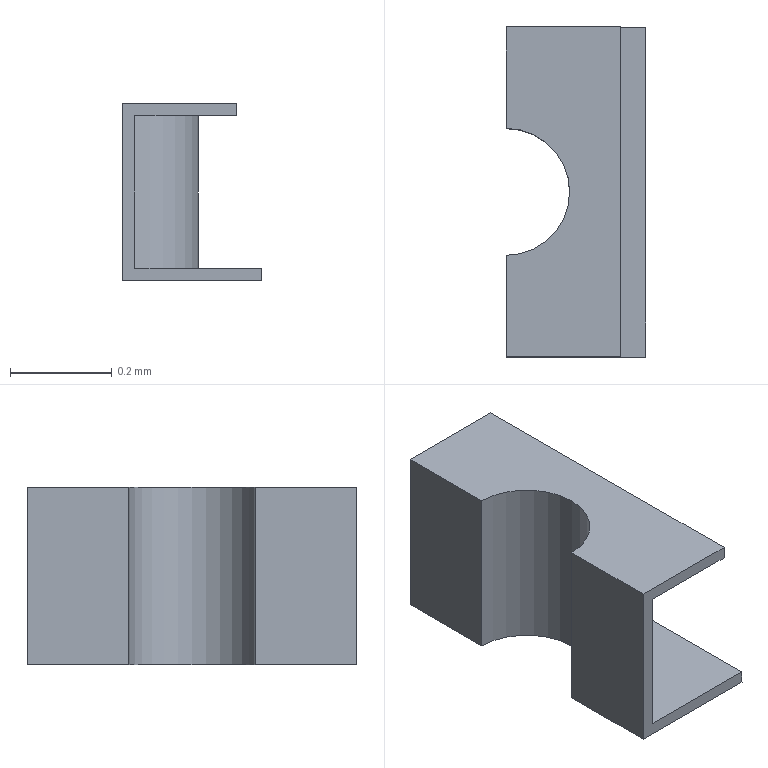Part | STEP file | RJ-USIO-V1_2-220411_91 | 1 solid | 14 faces | box 0.275 x 0.65 x 0.35 mm | volume 0.01277 mm3 | plane 12 | cylinder 2 | commonest cylinder face diameters 0.25 x1 0.3 x1
STEP:
#1=CARTESIAN_POINT('',(0.,0.,0.));
#2=DIRECTION('',(0.,0.,1.));
#3=DIRECTION('',(1.,0.,0.));
#4=AXIS2_PLACEMENT_3D('',#1,#2,#3);
#5=CARTESIAN_POINT('',(59.475,56.625,0.004766));
#6=VERTEX_POINT('',#5);
#7=CARTESIAN_POINT('',(59.475,56.825,0.004766));
#8=VERTEX_POINT('',#7);
#9=CARTESIAN_POINT('',(59.475,56.625,0.004766));
#10=DIRECTION('',(-0.000000044,1.,0.));
#11=VECTOR('',#10,1.);
#12=LINE('',#9,#11);
#13=CARTESIAN_POINT('',(59.55,56.5,0.004766));
#14=DIRECTION('',(0.,0.,1.));
#15=DIRECTION('',(0.000000044,-1.,0.));
#16=AXIS2_PLACEMENT_3D('',#13,#14,#15);
#17=PLANE('',#16);
#18=CARTESIAN_POINT('',(-0.125,-0.07522));
#19=DIRECTION('',(-1.,0.));
#20=VECTOR('',#19,1.);
#21=LINE('',#18,#20);
#22=(GEOMETRIC_REPRESENTATION_CONTEXT(2)PARAMETRIC_REPRESENTATION_CONTEXT()REPRESENTATION_CONTEXT('',''));
#23=DEFINITIONAL_REPRESENTATION('',(#21),#22);
#24=PCURVE('',#17,#23);
#25=CARTESIAN_POINT('',(59.475,56.65,0.004766));
#26=DIRECTION('',(-1.,-0.000000044,0.));
#27=DIRECTION('',(-0.000000044,1.,0.));
#28=AXIS2_PLACEMENT_3D('',#25,#26,#27);
#29=PLANE('',#28);
#30=CARTESIAN_POINT('',(-0.025,0.));
#31=DIRECTION('',(1.,0.));
#32=VECTOR('',#31,1.);
#33=LINE('',#30,#32);
#34=(GEOMETRIC_REPRESENTATION_CONTEXT(2)PARAMETRIC_REPRESENTATION_CONTEXT()REPRESENTATION_CONTEXT('',''));
#35=DEFINITIONAL_REPRESENTATION('',(#33),#34);
#36=PCURVE('',#29,#35);
#37=SURFACE_CURVE('',#12,(#24,#36),.PCURVE_S1.);
#38=EDGE_CURVE('',#6,#8,#37,.T.);
#39=ORIENTED_EDGE('',*,*,#38,.F.);
#40=CARTESIAN_POINT('',(59.475,56.375,0.004766));
#41=VERTEX_POINT('',#40);
#42=CARTESIAN_POINT('',(59.475,56.5,0.004766));
#43=DIRECTION('',(0.,0.,1.));
#44=DIRECTION('',(0.000000044,-1.,0.));
#45=AXIS2_PLACEMENT_3D('',#42,#43,#44);
#46=CIRCLE('',#45,0.125);
#47=CARTESIAN_POINT('',(0.,-0.07522));
#48=DIRECTION('',(1.,0.));
#49=AXIS2_PLACEMENT_2D('',#47,#48);
#50=CIRCLE('',#49,0.125);
#51=(GEOMETRIC_REPRESENTATION_CONTEXT(2)PARAMETRIC_REPRESENTATION_CONTEXT()REPRESENTATION_CONTEXT('',''));
#52=DEFINITIONAL_REPRESENTATION('',(#50),#51);
#53=PCURVE('',#17,#52);
#54=CARTESIAN_POINT('',(59.475,56.5,0.3548));
#55=DIRECTION('',(0.,0.,-1.));
#56=DIRECTION('',(-0.000000044,1.,0.));
#57=AXIS2_PLACEMENT_3D('',#54,#55,#56);
#58=CYLINDRICAL_SURFACE('',#57,0.125);
#59=CARTESIAN_POINT('',(3.142,0.35));
#60=DIRECTION('',(-1.,0.));
#61=VECTOR('',#60,1.);
#62=LINE('',#59,#61);
#63=(GEOMETRIC_REPRESENTATION_CONTEXT(2)PARAMETRIC_REPRESENTATION_CONTEXT()REPRESENTATION_CONTEXT('',''));
#64=DEFINITIONAL_REPRESENTATION('',(#62),#63);
#65=PCURVE('',#58,#64);
#66=SURFACE_CURVE('',#46,(#53,#65),.PCURVE_S1.);
#67=EDGE_CURVE('',#41,#6,#66,.T.);
#68=ORIENTED_EDGE('',*,*,#67,.F.);
#69=CARTESIAN_POINT('',(59.475,56.175,0.004766));
#70=VERTEX_POINT('',#69);
#71=CARTESIAN_POINT('',(59.475,56.175,0.004766));
#72=DIRECTION('',(-0.000000044,1.,0.));
#73=VECTOR('',#72,1.);
#74=LINE('',#71,#73);
#75=CARTESIAN_POINT('',(0.325,-0.07522));
#76=DIRECTION('',(-1.,0.));
#77=VECTOR('',#76,1.);
#78=LINE('',#75,#77);
#79=(GEOMETRIC_REPRESENTATION_CONTEXT(2)PARAMETRIC_REPRESENTATION_CONTEXT()REPRESENTATION_CONTEXT('',''));
#80=DEFINITIONAL_REPRESENTATION('',(#78),#79);
#81=PCURVE('',#17,#80);
#82=CARTESIAN_POINT('',(59.475,56.375,0.004766));
#83=DIRECTION('',(-1.,-0.000000044,0.));
#84=DIRECTION('',(-0.000000044,1.,0.));
#85=AXIS2_PLACEMENT_3D('',#82,#83,#84);
#86=PLANE('',#85);
#87=CARTESIAN_POINT('',(-0.2,0.));
#88=DIRECTION('',(1.,0.));
#89=VECTOR('',#88,1.);
#90=LINE('',#87,#89);
#91=(GEOMETRIC_REPRESENTATION_CONTEXT(2)PARAMETRIC_REPRESENTATION_CONTEXT()REPRESENTATION_CONTEXT('',''));
#92=DEFINITIONAL_REPRESENTATION('',(#90),#91);
#93=PCURVE('',#86,#92);
#94=SURFACE_CURVE('',#74,(#81,#93),.PCURVE_S1.);
#95=EDGE_CURVE('',#70,#41,#94,.T.);
#96=ORIENTED_EDGE('',*,*,#95,.F.);
#97=CARTESIAN_POINT('',(59.75,56.175,0.004766));
#98=VERTEX_POINT('',#97);
#99=CARTESIAN_POINT('',(59.75,56.175,0.004766));
#100=DIRECTION('',(-1.,-0.000000044,0.));
#101=VECTOR('',#100,1.);
#102=LINE('',#99,#101);
#103=CARTESIAN_POINT('',(0.325,0.1998));
#104=DIRECTION('',(0.,-1.));
#105=VECTOR('',#104,1.);
#106=LINE('',#103,#105);
#107=(GEOMETRIC_REPRESENTATION_CONTEXT(2)PARAMETRIC_REPRESENTATION_CONTEXT()REPRESENTATION_CONTEXT('',''));
#108=DEFINITIONAL_REPRESENTATION('',(#106),#107);
#109=PCURVE('',#17,#108);
#110=CARTESIAN_POINT('',(59.75,56.175,0.3298));
#111=DIRECTION('',(0.000000044,-1.,0.));
#112=DIRECTION('',(-1.,-0.000000044,0.));
#113=AXIS2_PLACEMENT_3D('',#110,#111,#112);
#114=PLANE('',#113);
#115=CARTESIAN_POINT('',(0.,0.325));
#116=DIRECTION('',(1.,0.));
#117=VECTOR('',#116,1.);
#118=LINE('',#115,#117);
#119=(GEOMETRIC_REPRESENTATION_CONTEXT(2)PARAMETRIC_REPRESENTATION_CONTEXT()REPRESENTATION_CONTEXT('',''));
#120=DEFINITIONAL_REPRESENTATION('',(#118),#119);
#121=PCURVE('',#114,#120);
#122=SURFACE_CURVE('',#102,(#109,#121),.PCURVE_S1.);
#123=EDGE_CURVE('',#98,#70,#122,.T.);
#124=ORIENTED_EDGE('',*,*,#123,.F.);
#125=CARTESIAN_POINT('',(59.75,56.825,0.004766));
#126=VERTEX_POINT('',#125);
#127=CARTESIAN_POINT('',(59.75,56.825,0.004766));
#128=DIRECTION('',(0.000000044,-1.,0.));
#129=VECTOR('',#128,1.);
#130=LINE('',#127,#129);
#131=CARTESIAN_POINT('',(-0.325,0.1998));
#132=DIRECTION('',(1.,0.));
#133=VECTOR('',#132,1.);
#134=LINE('',#131,#133);
#135=(GEOMETRIC_REPRESENTATION_CONTEXT(2)PARAMETRIC_REPRESENTATION_CONTEXT()REPRESENTATION_CONTEXT('',''));
#136=DEFINITIONAL_REPRESENTATION('',(#134),#135);
#137=PCURVE('',#17,#136);
#138=CARTESIAN_POINT('',(59.75,56.175,0.004766));
#139=DIRECTION('',(1.,0.000000044,0.));
#140=DIRECTION('',(0.000000044,-1.,0.));
#141=AXIS2_PLACEMENT_3D('',#138,#139,#140);
#142=PLANE('',#141);
#143=CARTESIAN_POINT('',(-0.65,0.));
#144=DIRECTION('',(1.,0.));
#145=VECTOR('',#144,1.);
#146=LINE('',#143,#145);
#147=(GEOMETRIC_REPRESENTATION_CONTEXT(2)PARAMETRIC_REPRESENTATION_CONTEXT()REPRESENTATION_CONTEXT('',''));
#148=DEFINITIONAL_REPRESENTATION('',(#146),#147);
#149=PCURVE('',#142,#148);
#150=SURFACE_CURVE('',#130,(#137,#149),.PCURVE_S1.);
#151=EDGE_CURVE('',#126,#98,#150,.T.);
#152=ORIENTED_EDGE('',*,*,#151,.F.);
#153=CARTESIAN_POINT('',(59.475,56.825,0.004766));
#154=DIRECTION('',(1.,0.000000044,0.));
#155=VECTOR('',#154,1.);
#156=LINE('',#153,#155);
#157=CARTESIAN_POINT('',(-0.325,-0.07522));
#158=DIRECTION('',(0.,1.));
#159=VECTOR('',#158,1.);
#160=LINE('',#157,#159);
#161=(GEOMETRIC_REPRESENTATION_CONTEXT(2)PARAMETRIC_REPRESENTATION_CONTEXT()REPRESENTATION_CONTEXT('',''));
#162=DEFINITIONAL_REPRESENTATION('',(#160),#161);
#163=PCURVE('',#17,#162);
#164=CARTESIAN_POINT('',(59.75,56.825,0.3548));
#165=DIRECTION('',(-0.000000044,1.,0.));
#166=DIRECTION('',(1.,0.000000044,0.));
#167=AXIS2_PLACEMENT_3D('',#164,#165,#166);
#168=PLANE('',#167);
#169=CARTESIAN_POINT('',(-0.275,0.35));
#170=DIRECTION('',(1.,0.));
#171=VECTOR('',#170,1.);
#172=LINE('',#169,#171);
#173=(GEOMETRIC_REPRESENTATION_CONTEXT(2)PARAMETRIC_REPRESENTATION_CONTEXT()REPRESENTATION_CONTEXT('',''));
#174=DEFINITIONAL_REPRESENTATION('',(#172),#173);
#175=PCURVE('',#168,#174);
#176=SURFACE_CURVE('',#156,(#163,#175),.PCURVE_S1.);
#177=EDGE_CURVE('',#8,#126,#176,.T.);
#178=ORIENTED_EDGE('',*,*,#177,.F.);
#179=EDGE_LOOP('',(#39,#68,#96,#124,#152,#178));
#180=FACE_BOUND('',#179,.F.);
#181=ADVANCED_FACE('',(#180),#17,.F.);
#182=CARTESIAN_POINT('',(59.475,56.825,0.3548));
#183=VERTEX_POINT('',#182);
#184=CARTESIAN_POINT('',(59.475,56.625,0.3548));
#185=VERTEX_POINT('',#184);
#186=CARTESIAN_POINT('',(59.475,56.825,0.3548));
#187=DIRECTION('',(0.000000044,-1.,0.));
#188=VECTOR('',#187,1.);
#189=LINE('',#186,#188);
#190=CARTESIAN_POINT('',(0.175,-0.35));
#191=DIRECTION('',(-1.,0.));
#192=VECTOR('',#191,1.);
#193=LINE('',#190,#192);
#194=(GEOMETRIC_REPRESENTATION_CONTEXT(2)PARAMETRIC_REPRESENTATION_CONTEXT()REPRESENTATION_CONTEXT('',''));
#195=DEFINITIONAL_REPRESENTATION('',(#193),#194);
#196=PCURVE('',#29,#195);
#197=CARTESIAN_POINT('',(59.75,56.175,0.3548));
#198=DIRECTION('',(0.,0.,1.));
#199=DIRECTION('',(0.000000044,-1.,0.));
#200=AXIS2_PLACEMENT_3D('',#197,#198,#199);
#201=PLANE('',#200);
#202=CARTESIAN_POINT('',(-0.65,-0.275));
#203=DIRECTION('',(1.,0.));
#204=VECTOR('',#203,1.);
#205=LINE('',#202,#204);
#206=(GEOMETRIC_REPRESENTATION_CONTEXT(2)PARAMETRIC_REPRESENTATION_CONTEXT()REPRESENTATION_CONTEXT('',''));
#207=DEFINITIONAL_REPRESENTATION('',(#205),#206);
#208=PCURVE('',#201,#207);
#209=SURFACE_CURVE('',#189,(#196,#208),.PCURVE_S1.);
#210=EDGE_CURVE('',#183,#185,#209,.T.);
#211=ORIENTED_EDGE('',*,*,#210,.T.);
#212=CARTESIAN_POINT('',(59.475,56.625,0.3548));
#213=DIRECTION('',(0.,0.,-1.));
#214=VECTOR('',#213,1.);
#215=LINE('',#212,#214);
#216=CARTESIAN_POINT('',(-0.025,-0.35));
#217=DIRECTION('',(0.,1.));
#218=VECTOR('',#217,1.);
#219=LINE('',#216,#218);
#220=(GEOMETRIC_REPRESENTATION_CONTEXT(2)PARAMETRIC_REPRESENTATION_CONTEXT()REPRESENTATION_CONTEXT('',''));
#221=DEFINITIONAL_REPRESENTATION('',(#219),#220);
#222=PCURVE('',#29,#221);
#223=CARTESIAN_POINT('',(0.,0.));
#224=DIRECTION('',(0.,1.));
#225=VECTOR('',#224,1.);
#226=LINE('',#223,#225);
#227=(GEOMETRIC_REPRESENTATION_CONTEXT(2)PARAMETRIC_REPRESENTATION_CONTEXT()REPRESENTATION_CONTEXT('',''));
#228=DEFINITIONAL_REPRESENTATION('',(#226),#227);
#229=PCURVE('',#58,#228);
#230=SURFACE_CURVE('',#215,(#222,#229),.PCURVE_S1.);
#231=EDGE_CURVE('',#185,#6,#230,.T.);
#232=ORIENTED_EDGE('',*,*,#231,.T.);
#233=ORIENTED_EDGE('',*,*,#38,.T.);
#234=CARTESIAN_POINT('',(59.475,56.825,0.004766));
#235=DIRECTION('',(0.,0.,1.));
#236=VECTOR('',#235,1.);
#237=LINE('',#234,#236);
#238=CARTESIAN_POINT('',(0.175,0.));
#239=DIRECTION('',(0.,-1.));
#240=VECTOR('',#239,1.);
#241=LINE('',#238,#240);
#242=(GEOMETRIC_REPRESENTATION_CONTEXT(2)PARAMETRIC_REPRESENTATION_CONTEXT()REPRESENTATION_CONTEXT('',''));
#243=DEFINITIONAL_REPRESENTATION('',(#241),#242);
#244=PCURVE('',#29,#243);
#245=CARTESIAN_POINT('',(-0.275,0.35));
#246=DIRECTION('',(0.,-1.));
#247=VECTOR('',#246,1.);
#248=LINE('',#245,#247);
#249=(GEOMETRIC_REPRESENTATION_CONTEXT(2)PARAMETRIC_REPRESENTATION_CONTEXT()REPRESENTATION_CONTEXT('',''));
#250=DEFINITIONAL_REPRESENTATION('',(#248),#249);
#251=PCURVE('',#168,#250);
#252=SURFACE_CURVE('',#237,(#244,#251),.PCURVE_S1.);
#253=EDGE_CURVE('',#8,#183,#252,.T.);
#254=ORIENTED_EDGE('',*,*,#253,.T.);
#255=EDGE_LOOP('',(#211,#232,#233,#254));
#256=FACE_BOUND('',#255,.F.);
#257=ADVANCED_FACE('',(#256),#29,.T.);
#258=ORIENTED_EDGE('',*,*,#210,.F.);
#259=CARTESIAN_POINT('',(59.7,56.825,0.3548));
#260=VERTEX_POINT('',#259);
#261=CARTESIAN_POINT('',(59.7,56.825,0.3548));
#262=DIRECTION('',(-1.,-0.000000044,0.));
#263=VECTOR('',#262,1.);
#264=LINE('',#261,#263);
#265=CARTESIAN_POINT('',(-0.65,-0.05));
#266=DIRECTION('',(0.,-1.));
#267=VECTOR('',#266,1.);
#268=LINE('',#265,#267);
#269=(GEOMETRIC_REPRESENTATION_CONTEXT(2)PARAMETRIC_REPRESENTATION_CONTEXT()REPRESENTATION_CONTEXT('',''));
#270=DEFINITIONAL_REPRESENTATION('',(#268),#269);
#271=PCURVE('',#201,#270);
#272=CARTESIAN_POINT('',(-0.05,0.));
#273=DIRECTION('',(-1.,0.));
#274=VECTOR('',#273,1.);
#275=LINE('',#272,#274);
#276=(GEOMETRIC_REPRESENTATION_CONTEXT(2)PARAMETRIC_REPRESENTATION_CONTEXT()REPRESENTATION_CONTEXT('',''));
#277=DEFINITIONAL_REPRESENTATION('',(#275),#276);
#278=PCURVE('',#168,#277);
#279=SURFACE_CURVE('',#264,(#271,#278),.PCURVE_S1.);
#280=EDGE_CURVE('',#260,#183,#279,.T.);
#281=ORIENTED_EDGE('',*,*,#280,.F.);
#282=CARTESIAN_POINT('',(59.7,56.175,0.3548));
#283=VERTEX_POINT('',#282);
#284=CARTESIAN_POINT('',(59.7,56.825,0.3548));
#285=DIRECTION('',(0.000000044,-1.,0.));
#286=VECTOR('',#285,1.);
#287=LINE('',#284,#286);
#288=CARTESIAN_POINT('',(-0.65,-0.05));
#289=DIRECTION('',(1.,0.));
#290=VECTOR('',#289,1.);
#291=LINE('',#288,#290);
#292=(GEOMETRIC_REPRESENTATION_CONTEXT(2)PARAMETRIC_REPRESENTATION_CONTEXT()REPRESENTATION_CONTEXT('',''));
#293=DEFINITIONAL_REPRESENTATION('',(#291),#292);
#294=PCURVE('',#201,#293);
#295=CARTESIAN_POINT('',(59.7,56.5,0.3423));
#296=DIRECTION('',(1.,0.000000044,0.));
#297=DIRECTION('',(0.000000044,-1.,0.));
#298=AXIS2_PLACEMENT_3D('',#295,#296,#297);
#299=PLANE('',#298);
#300=CARTESIAN_POINT('',(-0.325,-0.0125));
#301=DIRECTION('',(1.,0.));
#302=VECTOR('',#301,1.);
#303=LINE('',#300,#302);
#304=(GEOMETRIC_REPRESENTATION_CONTEXT(2)PARAMETRIC_REPRESENTATION_CONTEXT()REPRESENTATION_CONTEXT('',''));
#305=DEFINITIONAL_REPRESENTATION('',(#303),#304);
#306=PCURVE('',#299,#305);
#307=SURFACE_CURVE('',#287,(#294,#306),.PCURVE_S1.);
#308=EDGE_CURVE('',#260,#283,#307,.T.);
#309=ORIENTED_EDGE('',*,*,#308,.T.);
#310=CARTESIAN_POINT('',(59.475,56.175,0.3548));
#311=VERTEX_POINT('',#310);
#312=CARTESIAN_POINT('',(59.475,56.175,0.3548));
#313=DIRECTION('',(1.,0.000000044,0.));
#314=VECTOR('',#313,1.);
#315=LINE('',#312,#314);
#316=CARTESIAN_POINT('',(0.,-0.275));
#317=DIRECTION('',(0.,1.));
#318=VECTOR('',#317,1.);
#319=LINE('',#316,#318);
#320=(GEOMETRIC_REPRESENTATION_CONTEXT(2)PARAMETRIC_REPRESENTATION_CONTEXT()REPRESENTATION_CONTEXT('',''));
#321=DEFINITIONAL_REPRESENTATION('',(#319),#320);
#322=PCURVE('',#201,#321);
#323=CARTESIAN_POINT('',(0.275,-0.025));
#324=DIRECTION('',(-1.,0.));
#325=VECTOR('',#324,1.);
#326=LINE('',#323,#325);
#327=(GEOMETRIC_REPRESENTATION_CONTEXT(2)PARAMETRIC_REPRESENTATION_CONTEXT()REPRESENTATION_CONTEXT('',''));
#328=DEFINITIONAL_REPRESENTATION('',(#326),#327);
#329=PCURVE('',#114,#328);
#330=SURFACE_CURVE('',#315,(#322,#329),.PCURVE_S1.);
#331=EDGE_CURVE('',#311,#283,#330,.T.);
#332=ORIENTED_EDGE('',*,*,#331,.F.);
#333=CARTESIAN_POINT('',(59.475,56.375,0.3548));
#334=VERTEX_POINT('',#333);
#335=CARTESIAN_POINT('',(59.475,56.375,0.3548));
#336=DIRECTION('',(0.000000044,-1.,0.));
#337=VECTOR('',#336,1.);
#338=LINE('',#335,#337);
#339=CARTESIAN_POINT('',(-0.2,-0.275));
#340=DIRECTION('',(1.,0.));
#341=VECTOR('',#340,1.);
#342=LINE('',#339,#341);
#343=(GEOMETRIC_REPRESENTATION_CONTEXT(2)PARAMETRIC_REPRESENTATION_CONTEXT()REPRESENTATION_CONTEXT('',''));
#344=DEFINITIONAL_REPRESENTATION('',(#342),#343);
#345=PCURVE('',#201,#344);
#346=CARTESIAN_POINT('',(0.,-0.35));
#347=DIRECTION('',(-1.,0.));
#348=VECTOR('',#347,1.);
#349=LINE('',#346,#348);
#350=(GEOMETRIC_REPRESENTATION_CONTEXT(2)PARAMETRIC_REPRESENTATION_CONTEXT()REPRESENTATION_CONTEXT('',''));
#351=DEFINITIONAL_REPRESENTATION('',(#349),#350);
#352=PCURVE('',#86,#351);
#353=SURFACE_CURVE('',#338,(#345,#352),.PCURVE_S1.);
#354=EDGE_CURVE('',#334,#311,#353,.T.);
#355=ORIENTED_EDGE('',*,*,#354,.F.);
#356=CARTESIAN_POINT('',(59.475,56.5,0.3548));
#357=DIRECTION('',(0.,0.,-1.));
#358=DIRECTION('',(-0.000000044,1.,0.));
#359=AXIS2_PLACEMENT_3D('',#356,#357,#358);
#360=CIRCLE('',#359,0.125);
#361=CARTESIAN_POINT('',(-0.45,-0.275));
#362=CARTESIAN_POINT('',(-0.45,-0.05849));
#363=CARTESIAN_POINT('',(-0.2625,-0.1667));
#364=CARTESIAN_POINT('',(-0.075,-0.275));
#365=CARTESIAN_POINT('',(-0.2625,-0.3833));
#366=CARTESIAN_POINT('',(-0.45,-0.4915));
#367=CARTESIAN_POINT('',(-0.45,-0.275));
#368=(BOUNDED_CURVE()B_SPLINE_CURVE(2,(#361,#362,#363,#364,#365,#366,#367),.UNSPECIFIED.,.T.,.F.)B_SPLINE_CURVE_WITH_KNOTS((1,2,2,2,2,1),(-2.094,0.,2.094,4.189,6.283,8.378),.UNSPECIFIED.)CURVE()GEOMETRIC_REPRESENTATION_ITEM()RATIONAL_B_SPLINE_CURVE((1.,0.5,1.,0.5,1.,0.5,1.))REPRESENTATION_ITEM(''));
#369=(GEOMETRIC_REPRESENTATION_CONTEXT(2)PARAMETRIC_REPRESENTATION_CONTEXT()REPRESENTATION_CONTEXT('',''));
#370=DEFINITIONAL_REPRESENTATION('',(#368),#369);
#371=PCURVE('',#201,#370);
#372=CARTESIAN_POINT('',(0.,0.));
#373=DIRECTION('',(1.,0.));
#374=VECTOR('',#373,1.);
#375=LINE('',#372,#374);
#376=(GEOMETRIC_REPRESENTATION_CONTEXT(2)PARAMETRIC_REPRESENTATION_CONTEXT()REPRESENTATION_CONTEXT('',''));
#377=DEFINITIONAL_REPRESENTATION('',(#375),#376);
#378=PCURVE('',#58,#377);
#379=SURFACE_CURVE('',#360,(#371,#378),.PCURVE_S1.);
#380=EDGE_CURVE('',#185,#334,#379,.T.);
#381=ORIENTED_EDGE('',*,*,#380,.F.);
#382=EDGE_LOOP('',(#258,#281,#309,#332,#355,#381));
#383=FACE_BOUND('',#382,.F.);
#384=ADVANCED_FACE('',(#383),#201,.T.);
#385=CARTESIAN_POINT('',(59.75,56.825,0.02977));
#386=VERTEX_POINT('',#385);
#387=CARTESIAN_POINT('',(59.75,56.825,0.004766));
#388=DIRECTION('',(0.,0.,1.));
#389=VECTOR('',#388,1.);
#390=LINE('',#387,#389);
#391=CARTESIAN_POINT('',(0.,0.35));
#392=DIRECTION('',(0.,-1.));
#393=VECTOR('',#392,1.);
#394=LINE('',#391,#393);
#395=(GEOMETRIC_REPRESENTATION_CONTEXT(2)PARAMETRIC_REPRESENTATION_CONTEXT()REPRESENTATION_CONTEXT('',''));
#396=DEFINITIONAL_REPRESENTATION('',(#394),#395);
#397=PCURVE('',#168,#396);
#398=CARTESIAN_POINT('',(-0.65,0.));
#399=DIRECTION('',(0.,-1.));
#400=VECTOR('',#399,1.);
#401=LINE('',#398,#400);
#402=(GEOMETRIC_REPRESENTATION_CONTEXT(2)PARAMETRIC_REPRESENTATION_CONTEXT()REPRESENTATION_CONTEXT('',''));
#403=DEFINITIONAL_REPRESENTATION('',(#401),#402);
#404=PCURVE('',#142,#403);
#405=SURFACE_CURVE('',#390,(#397,#404),.PCURVE_S1.);
#406=EDGE_CURVE('',#126,#386,#405,.T.);
#407=ORIENTED_EDGE('',*,*,#406,.T.);
#408=CARTESIAN_POINT('',(59.5,56.825,0.02977));
#409=VERTEX_POINT('',#408);
#410=CARTESIAN_POINT('',(59.75,56.825,0.02977));
#411=DIRECTION('',(-1.,-0.000000044,0.));
#412=VECTOR('',#411,1.);
#413=LINE('',#410,#412);
#414=CARTESIAN_POINT('',(0.,0.325));
#415=DIRECTION('',(-1.,0.));
#416=VECTOR('',#415,1.);
#417=LINE('',#414,#416);
#418=(GEOMETRIC_REPRESENTATION_CONTEXT(2)PARAMETRIC_REPRESENTATION_CONTEXT()REPRESENTATION_CONTEXT('',''));
#419=DEFINITIONAL_REPRESENTATION('',(#417),#418);
#420=PCURVE('',#168,#419);
#421=CARTESIAN_POINT('',(59.625,56.5,0.02977));
#422=DIRECTION('',(0.,0.,1.));
#423=DIRECTION('',(0.000000044,-1.,0.));
#424=AXIS2_PLACEMENT_3D('',#421,#422,#423);
#425=PLANE('',#424);
#426=CARTESIAN_POINT('',(-0.325,0.125));
#427=DIRECTION('',(0.,-1.));
#428=VECTOR('',#427,1.);
#429=LINE('',#426,#428);
#430=(GEOMETRIC_REPRESENTATION_CONTEXT(2)PARAMETRIC_REPRESENTATION_CONTEXT()REPRESENTATION_CONTEXT('',''));
#431=DEFINITIONAL_REPRESENTATION('',(#429),#430);
#432=PCURVE('',#425,#431);
#433=SURFACE_CURVE('',#413,(#420,#432),.PCURVE_S1.);
#434=EDGE_CURVE('',#386,#409,#433,.T.);
#435=ORIENTED_EDGE('',*,*,#434,.T.);
#436=CARTESIAN_POINT('',(59.5,56.825,0.3298));
#437=VERTEX_POINT('',#436);
#438=CARTESIAN_POINT('',(59.5,56.825,0.02977));
#439=DIRECTION('',(0.,0.,1.));
#440=VECTOR('',#439,1.);
#441=LINE('',#438,#440);
#442=CARTESIAN_POINT('',(-0.25,0.325));
#443=DIRECTION('',(0.,-1.));
#444=VECTOR('',#443,1.);
#445=LINE('',#442,#444);
#446=(GEOMETRIC_REPRESENTATION_CONTEXT(2)PARAMETRIC_REPRESENTATION_CONTEXT()REPRESENTATION_CONTEXT('',''));
#447=DEFINITIONAL_REPRESENTATION('',(#445),#446);
#448=PCURVE('',#168,#447);
#449=CARTESIAN_POINT('',(59.5,56.825,0.3298));
#450=DIRECTION('',(1.,0.000000044,0.));
#451=DIRECTION('',(0.000000044,-1.,0.));
#452=AXIS2_PLACEMENT_3D('',#449,#450,#451);
#453=PLANE('',#452);
#454=CARTESIAN_POINT('',(0.,0.3));
#455=DIRECTION('',(0.,-1.));
#456=VECTOR('',#455,1.);
#457=LINE('',#454,#456);
#458=(GEOMETRIC_REPRESENTATION_CONTEXT(2)PARAMETRIC_REPRESENTATION_CONTEXT()REPRESENTATION_CONTEXT('',''));
#459=DEFINITIONAL_REPRESENTATION('',(#457),#458);
#460=PCURVE('',#453,#459);
#461=SURFACE_CURVE('',#441,(#448,#460),.PCURVE_S1.);
#462=EDGE_CURVE('',#409,#437,#461,.T.);
#463=ORIENTED_EDGE('',*,*,#462,.T.);
#464=CARTESIAN_POINT('',(59.7,56.825,0.3298));
#465=VERTEX_POINT('',#464);
#466=CARTESIAN_POINT('',(59.5,56.825,0.3298));
#467=DIRECTION('',(1.,0.000000044,0.));
#468=VECTOR('',#467,1.);
#469=LINE('',#466,#468);
#470=CARTESIAN_POINT('',(-0.25,0.025));
#471=DIRECTION('',(1.,0.));
#472=VECTOR('',#471,1.);
#473=LINE('',#470,#472);
#474=(GEOMETRIC_REPRESENTATION_CONTEXT(2)PARAMETRIC_REPRESENTATION_CONTEXT()REPRESENTATION_CONTEXT('',''));
#475=DEFINITIONAL_REPRESENTATION('',(#473),#474);
#476=PCURVE('',#168,#475);
#477=CARTESIAN_POINT('',(59.75,56.825,0.3298));
#478=DIRECTION('',(0.,0.,-1.));
#479=DIRECTION('',(-0.000000044,1.,0.));
#480=AXIS2_PLACEMENT_3D('',#477,#478,#479);
#481=PLANE('',#480);
#482=CARTESIAN_POINT('',(0.,-0.25));
#483=DIRECTION('',(0.,1.));
#484=VECTOR('',#483,1.);
#485=LINE('',#482,#484);
#486=(GEOMETRIC_REPRESENTATION_CONTEXT(2)PARAMETRIC_REPRESENTATION_CONTEXT()REPRESENTATION_CONTEXT('',''));
#487=DEFINITIONAL_REPRESENTATION('',(#485),#486);
#488=PCURVE('',#481,#487);
#489=SURFACE_CURVE('',#469,(#476,#488),.PCURVE_S1.);
#490=EDGE_CURVE('',#437,#465,#489,.T.);
#491=ORIENTED_EDGE('',*,*,#490,.T.);
#492=CARTESIAN_POINT('',(59.7,56.825,0.3298));
#493=DIRECTION('',(0.,0.,1.));
#494=VECTOR('',#493,1.);
#495=LINE('',#492,#494);
#496=CARTESIAN_POINT('',(-0.05,0.025));
#497=DIRECTION('',(0.,-1.));
#498=VECTOR('',#497,1.);
#499=LINE('',#496,#498);
#500=(GEOMETRIC_REPRESENTATION_CONTEXT(2)PARAMETRIC_REPRESENTATION_CONTEXT()REPRESENTATION_CONTEXT('',''));
#501=DEFINITIONAL_REPRESENTATION('',(#499),#500);
#502=PCURVE('',#168,#501);
#503=CARTESIAN_POINT('',(-0.325,0.0125));
#504=DIRECTION('',(0.,-1.));
#505=VECTOR('',#504,1.);
#506=LINE('',#503,#505);
#507=(GEOMETRIC_REPRESENTATION_CONTEXT(2)PARAMETRIC_REPRESENTATION_CONTEXT()REPRESENTATION_CONTEXT('',''));
#508=DEFINITIONAL_REPRESENTATION('',(#506),#507);
#509=PCURVE('',#299,#508);
#510=SURFACE_CURVE('',#495,(#502,#509),.PCURVE_S1.);
#511=EDGE_CURVE('',#465,#260,#510,.T.);
#512=ORIENTED_EDGE('',*,*,#511,.T.);
#513=ORIENTED_EDGE('',*,*,#280,.T.);
#514=ORIENTED_EDGE('',*,*,#253,.F.);
#515=ORIENTED_EDGE('',*,*,#177,.T.);
#516=EDGE_LOOP('',(#407,#435,#463,#491,#512,#513,#514,#515));
#517=FACE_BOUND('',#516,.F.);
#518=ADVANCED_FACE('',(#517),#168,.T.);
#519=CARTESIAN_POINT('',(59.75,56.175,0.02977));
#520=VERTEX_POINT('',#519);
#521=CARTESIAN_POINT('',(59.75,56.175,0.02977));
#522=DIRECTION('',(-0.000000044,1.,0.));
#523=VECTOR('',#522,1.);
#524=LINE('',#521,#523);
#525=CARTESIAN_POINT('',(0.,-0.025));
#526=DIRECTION('',(-1.,0.));
#527=VECTOR('',#526,1.);
#528=LINE('',#525,#527);
#529=(GEOMETRIC_REPRESENTATION_CONTEXT(2)PARAMETRIC_REPRESENTATION_CONTEXT()REPRESENTATION_CONTEXT('',''));
#530=DEFINITIONAL_REPRESENTATION('',(#528),#529);
#531=PCURVE('',#142,#530);
#532=CARTESIAN_POINT('',(0.325,0.125));
#533=DIRECTION('',(-1.,0.));
#534=VECTOR('',#533,1.);
#535=LINE('',#532,#534);
#536=(GEOMETRIC_REPRESENTATION_CONTEXT(2)PARAMETRIC_REPRESENTATION_CONTEXT()REPRESENTATION_CONTEXT('',''));
#537=DEFINITIONAL_REPRESENTATION('',(#535),#536);
#538=PCURVE('',#425,#537);
#539=SURFACE_CURVE('',#524,(#531,#538),.PCURVE_S1.);
#540=EDGE_CURVE('',#520,#386,#539,.T.);
#541=ORIENTED_EDGE('',*,*,#540,.T.);
#542=ORIENTED_EDGE('',*,*,#406,.F.);
#543=ORIENTED_EDGE('',*,*,#151,.T.);
#544=CARTESIAN_POINT('',(59.75,56.175,0.004766));
#545=DIRECTION('',(0.,0.,1.));
#546=VECTOR('',#545,1.);
#547=LINE('',#544,#546);
#548=CARTESIAN_POINT('',(0.,0.));
#549=DIRECTION('',(0.,-1.));
#550=VECTOR('',#549,1.);
#551=LINE('',#548,#550);
#552=(GEOMETRIC_REPRESENTATION_CONTEXT(2)PARAMETRIC_REPRESENTATION_CONTEXT()REPRESENTATION_CONTEXT('',''));
#553=DEFINITIONAL_REPRESENTATION('',(#551),#552);
#554=PCURVE('',#142,#553);
#555=CARTESIAN_POINT('',(0.,0.325));
#556=DIRECTION('',(0.,-1.));
#557=VECTOR('',#556,1.);
#558=LINE('',#555,#557);
#559=(GEOMETRIC_REPRESENTATION_CONTEXT(2)PARAMETRIC_REPRESENTATION_CONTEXT()REPRESENTATION_CONTEXT('',''));
#560=DEFINITIONAL_REPRESENTATION('',(#558),#559);
#561=PCURVE('',#114,#560);
#562=SURFACE_CURVE('',#547,(#554,#561),.PCURVE_S1.);
#563=EDGE_CURVE('',#98,#520,#562,.T.);
#564=ORIENTED_EDGE('',*,*,#563,.T.);
#565=EDGE_LOOP('',(#541,#542,#543,#564));
#566=FACE_BOUND('',#565,.F.);
#567=ADVANCED_FACE('',(#566),#142,.T.);
#568=CARTESIAN_POINT('',(59.5,56.175,0.02977));
#569=VERTEX_POINT('',#568);
#570=CARTESIAN_POINT('',(59.5,56.175,0.02977));
#571=DIRECTION('',(1.,0.000000044,0.));
#572=VECTOR('',#571,1.);
#573=LINE('',#570,#572);
#574=CARTESIAN_POINT('',(0.325,-0.125));
#575=DIRECTION('',(0.,1.));
#576=VECTOR('',#575,1.);
#577=LINE('',#574,#576);
#578=(GEOMETRIC_REPRESENTATION_CONTEXT(2)PARAMETRIC_REPRESENTATION_CONTEXT()REPRESENTATION_CONTEXT('',''));
#579=DEFINITIONAL_REPRESENTATION('',(#577),#578);
#580=PCURVE('',#425,#579);
#581=CARTESIAN_POINT('',(0.25,0.3));
#582=DIRECTION('',(-1.,0.));
#583=VECTOR('',#582,1.);
#584=LINE('',#581,#583);
#585=(GEOMETRIC_REPRESENTATION_CONTEXT(2)PARAMETRIC_REPRESENTATION_CONTEXT()REPRESENTATION_CONTEXT('',''));
#586=DEFINITIONAL_REPRESENTATION('',(#584),#585);
#587=PCURVE('',#114,#586);
#588=SURFACE_CURVE('',#573,(#580,#587),.PCURVE_S1.);
#589=EDGE_CURVE('',#569,#520,#588,.T.);
#590=ORIENTED_EDGE('',*,*,#589,.F.);
#591=CARTESIAN_POINT('',(59.5,56.352,0.02977));
#592=VERTEX_POINT('',#591);
#593=CARTESIAN_POINT('',(59.5,56.175,0.02977));
#594=DIRECTION('',(-0.000000044,1.,0.));
#595=VECTOR('',#594,1.);
#596=LINE('',#593,#595);
#597=CARTESIAN_POINT('',(0.325,-0.125));
#598=DIRECTION('',(-1.,0.));
#599=VECTOR('',#598,1.);
#600=LINE('',#597,#599);
#601=(GEOMETRIC_REPRESENTATION_CONTEXT(2)PARAMETRIC_REPRESENTATION_CONTEXT()REPRESENTATION_CONTEXT('',''));
#602=DEFINITIONAL_REPRESENTATION('',(#600),#601);
#603=PCURVE('',#425,#602);
#604=CARTESIAN_POINT('',(59.5,56.825,0.3298));
#605=DIRECTION('',(1.,0.000000044,0.));
#606=DIRECTION('',(0.000000044,-1.,0.));
#607=AXIS2_PLACEMENT_3D('',#604,#605,#606);
#608=PLANE('',#607);
#609=CARTESIAN_POINT('',(0.65,0.3));
#610=DIRECTION('',(-1.,0.));
#611=VECTOR('',#610,1.);
#612=LINE('',#609,#611);
#613=(GEOMETRIC_REPRESENTATION_CONTEXT(2)PARAMETRIC_REPRESENTATION_CONTEXT()REPRESENTATION_CONTEXT('',''));
#614=DEFINITIONAL_REPRESENTATION('',(#612),#613);
#615=PCURVE('',#608,#614);
#616=SURFACE_CURVE('',#596,(#603,#615),.PCURVE_S1.);
#617=EDGE_CURVE('',#569,#592,#616,.T.);
#618=ORIENTED_EDGE('',*,*,#617,.T.);
#619=CARTESIAN_POINT('',(59.5,56.648,0.02977));
#620=VERTEX_POINT('',#619);
#621=CARTESIAN_POINT('',(59.475,56.5,0.02977));
#622=DIRECTION('',(0.,0.,-1.));
#623=DIRECTION('',(0.1667,0.986,0.));
#624=AXIS2_PLACEMENT_3D('',#621,#622,#623);
#625=CIRCLE('',#624,0.15);
#626=CARTESIAN_POINT('',(-0.1479,-0.125));
#627=CARTESIAN_POINT('',(-0.1046,0.1312));
#628=CARTESIAN_POINT('',(0.0956,-0.03441));
#629=CARTESIAN_POINT('',(0.2958,-0.2));
#630=CARTESIAN_POINT('',(0.0523,-0.2906));
#631=CARTESIAN_POINT('',(-0.1912,-0.3812));
#632=CARTESIAN_POINT('',(-0.1479,-0.125));
#633=(BOUNDED_CURVE()B_SPLINE_CURVE(2,(#626,#627,#628,#629,#630,#631,#632),.UNSPECIFIED.,.T.,.F.)B_SPLINE_CURVE_WITH_KNOTS((1,2,2,2,2,1),(-2.094,0.,2.094,4.189,6.283,8.378),.UNSPECIFIED.)CURVE()GEOMETRIC_REPRESENTATION_ITEM()RATIONAL_B_SPLINE_CURVE((1.,0.5,1.,0.5,1.,0.5,1.))REPRESENTATION_ITEM(''));
#634=(GEOMETRIC_REPRESENTATION_CONTEXT(2)PARAMETRIC_REPRESENTATION_CONTEXT()REPRESENTATION_CONTEXT('',''));
#635=DEFINITIONAL_REPRESENTATION('',(#633),#634);
#636=PCURVE('',#425,#635);
#637=CARTESIAN_POINT('',(59.475,56.5,0.004766));
#638=DIRECTION('',(0.,0.,-1.));
#639=DIRECTION('',(-0.000000044,1.,0.));
#640=AXIS2_PLACEMENT_3D('',#637,#638,#639);
#641=CYLINDRICAL_SURFACE('',#640,0.15);
#642=CARTESIAN_POINT('',(0.1674,-0.025));
#643=DIRECTION('',(1.,0.));
#644=VECTOR('',#643,1.);
#645=LINE('',#642,#644);
#646=(GEOMETRIC_REPRESENTATION_CONTEXT(2)PARAMETRIC_REPRESENTATION_CONTEXT()REPRESENTATION_CONTEXT('',''));
#647=DEFINITIONAL_REPRESENTATION('',(#645),#646);
#648=PCURVE('',#641,#647);
#649=SURFACE_CURVE('',#625,(#636,#648),.PCURVE_S1.);
#650=EDGE_CURVE('',#620,#592,#649,.T.);
#651=ORIENTED_EDGE('',*,*,#650,.F.);
#652=CARTESIAN_POINT('',(59.5,56.648,0.02977));
#653=DIRECTION('',(-0.000000044,1.,0.));
#654=VECTOR('',#653,1.);
#655=LINE('',#652,#654);
#656=CARTESIAN_POINT('',(-0.1479,-0.125));
#657=DIRECTION('',(-1.,0.));
#658=VECTOR('',#657,1.);
#659=LINE('',#656,#658);
#660=(GEOMETRIC_REPRESENTATION_CONTEXT(2)PARAMETRIC_REPRESENTATION_CONTEXT()REPRESENTATION_CONTEXT('',''));
#661=DEFINITIONAL_REPRESENTATION('',(#659),#660);
#662=PCURVE('',#425,#661);
#663=CARTESIAN_POINT('',(0.1771,0.3));
#664=DIRECTION('',(-1.,0.));
#665=VECTOR('',#664,1.);
#666=LINE('',#663,#665);
#667=(GEOMETRIC_REPRESENTATION_CONTEXT(2)PARAMETRIC_REPRESENTATION_CONTEXT()REPRESENTATION_CONTEXT('',''));
#668=DEFINITIONAL_REPRESENTATION('',(#666),#667);
#669=PCURVE('',#453,#668);
#670=SURFACE_CURVE('',#655,(#662,#669),.PCURVE_S1.);
#671=EDGE_CURVE('',#620,#409,#670,.T.);
#672=ORIENTED_EDGE('',*,*,#671,.T.);
#673=ORIENTED_EDGE('',*,*,#434,.F.);
#674=ORIENTED_EDGE('',*,*,#540,.F.);
#675=EDGE_LOOP('',(#590,#618,#651,#672,#673,#674));
#676=FACE_BOUND('',#675,.F.);
#677=ADVANCED_FACE('',(#676),#425,.T.);
#678=ORIENTED_EDGE('',*,*,#563,.F.);
#679=ORIENTED_EDGE('',*,*,#123,.T.);
#680=CARTESIAN_POINT('',(59.475,56.175,0.004766));
#681=DIRECTION('',(0.,0.,1.));
#682=VECTOR('',#681,1.);
#683=LINE('',#680,#682);
#684=CARTESIAN_POINT('',(0.275,0.325));
#685=DIRECTION('',(0.,-1.));
#686=VECTOR('',#685,1.);
#687=LINE('',#684,#686);
#688=(GEOMETRIC_REPRESENTATION_CONTEXT(2)PARAMETRIC_REPRESENTATION_CONTEXT()REPRESENTATION_CONTEXT('',''));
#689=DEFINITIONAL_REPRESENTATION('',(#687),#688);
#690=PCURVE('',#114,#689);
#691=CARTESIAN_POINT('',(-0.2,0.));
#692=DIRECTION('',(0.,-1.));
#693=VECTOR('',#692,1.);
#694=LINE('',#691,#693);
#695=(GEOMETRIC_REPRESENTATION_CONTEXT(2)PARAMETRIC_REPRESENTATION_CONTEXT()REPRESENTATION_CONTEXT('',''));
#696=DEFINITIONAL_REPRESENTATION('',(#694),#695);
#697=PCURVE('',#86,#696);
#698=SURFACE_CURVE('',#683,(#690,#697),.PCURVE_S1.);
#699=EDGE_CURVE('',#70,#311,#698,.T.);
#700=ORIENTED_EDGE('',*,*,#699,.T.);
#701=ORIENTED_EDGE('',*,*,#331,.T.);
#702=CARTESIAN_POINT('',(59.7,56.175,0.3298));
#703=VERTEX_POINT('',#702);
#704=CARTESIAN_POINT('',(59.7,56.175,0.3548));
#705=DIRECTION('',(0.,0.,-1.));
#706=VECTOR('',#705,1.);
#707=LINE('',#704,#706);
#708=CARTESIAN_POINT('',(0.05,-0.025));
#709=DIRECTION('',(0.,1.));
#710=VECTOR('',#709,1.);
#711=LINE('',#708,#710);
#712=(GEOMETRIC_REPRESENTATION_CONTEXT(2)PARAMETRIC_REPRESENTATION_CONTEXT()REPRESENTATION_CONTEXT('',''));
#713=DEFINITIONAL_REPRESENTATION('',(#711),#712);
#714=PCURVE('',#114,#713);
#715=CARTESIAN_POINT('',(0.325,-0.0125));
#716=DIRECTION('',(0.,1.));
#717=VECTOR('',#716,1.);
#718=LINE('',#715,#717);
#719=(GEOMETRIC_REPRESENTATION_CONTEXT(2)PARAMETRIC_REPRESENTATION_CONTEXT()REPRESENTATION_CONTEXT('',''));
#720=DEFINITIONAL_REPRESENTATION('',(#718),#719);
#721=PCURVE('',#299,#720);
#722=SURFACE_CURVE('',#707,(#714,#721),.PCURVE_S1.);
#723=EDGE_CURVE('',#283,#703,#722,.T.);
#724=ORIENTED_EDGE('',*,*,#723,.T.);
#725=CARTESIAN_POINT('',(59.5,56.175,0.3298));
#726=VERTEX_POINT('',#725);
#727=CARTESIAN_POINT('',(59.7,56.175,0.3298));
#728=DIRECTION('',(-1.,-0.000000044,0.));
#729=VECTOR('',#728,1.);
#730=LINE('',#727,#729);
#731=CARTESIAN_POINT('',(0.05,0.));
#732=DIRECTION('',(1.,0.));
#733=VECTOR('',#732,1.);
#734=LINE('',#731,#733);
#735=(GEOMETRIC_REPRESENTATION_CONTEXT(2)PARAMETRIC_REPRESENTATION_CONTEXT()REPRESENTATION_CONTEXT('',''));
#736=DEFINITIONAL_REPRESENTATION('',(#734),#735);
#737=PCURVE('',#114,#736);
#738=CARTESIAN_POINT('',(-0.65,-0.05));
#739=DIRECTION('',(0.,-1.));
#740=VECTOR('',#739,1.);
#741=LINE('',#738,#740);
#742=(GEOMETRIC_REPRESENTATION_CONTEXT(2)PARAMETRIC_REPRESENTATION_CONTEXT()REPRESENTATION_CONTEXT('',''));
#743=DEFINITIONAL_REPRESENTATION('',(#741),#742);
#744=PCURVE('',#481,#743);
#745=SURFACE_CURVE('',#730,(#737,#744),.PCURVE_S1.);
#746=EDGE_CURVE('',#703,#726,#745,.T.);
#747=ORIENTED_EDGE('',*,*,#746,.T.);
#748=CARTESIAN_POINT('',(59.5,56.175,0.3298));
#749=DIRECTION('',(0.,0.,-1.));
#750=VECTOR('',#749,1.);
#751=LINE('',#748,#750);
#752=CARTESIAN_POINT('',(0.25,0.));
#753=DIRECTION('',(0.,1.));
#754=VECTOR('',#753,1.);
#755=LINE('',#752,#754);
#756=(GEOMETRIC_REPRESENTATION_CONTEXT(2)PARAMETRIC_REPRESENTATION_CONTEXT()REPRESENTATION_CONTEXT('',''));
#757=DEFINITIONAL_REPRESENTATION('',(#755),#756);
#758=PCURVE('',#114,#757);
#759=CARTESIAN_POINT('',(0.65,0.));
#760=DIRECTION('',(0.,1.));
#761=VECTOR('',#760,1.);
#762=LINE('',#759,#761);
#763=(GEOMETRIC_REPRESENTATION_CONTEXT(2)PARAMETRIC_REPRESENTATION_CONTEXT()REPRESENTATION_CONTEXT('',''));
#764=DEFINITIONAL_REPRESENTATION('',(#762),#763);
#765=PCURVE('',#608,#764);
#766=SURFACE_CURVE('',#751,(#758,#765),.PCURVE_S1.);
#767=EDGE_CURVE('',#726,#569,#766,.T.);
#768=ORIENTED_EDGE('',*,*,#767,.T.);
#769=ORIENTED_EDGE('',*,*,#589,.T.);
#770=EDGE_LOOP('',(#678,#679,#700,#701,#724,#747,#768,#769));
#771=FACE_BOUND('',#770,.F.);
#772=ADVANCED_FACE('',(#771),#114,.T.);
#773=ORIENTED_EDGE('',*,*,#354,.T.);
#774=ORIENTED_EDGE('',*,*,#699,.F.);
#775=ORIENTED_EDGE('',*,*,#95,.T.);
#776=CARTESIAN_POINT('',(59.475,56.375,0.004766));
#777=DIRECTION('',(0.,0.,1.));
#778=VECTOR('',#777,1.);
#779=LINE('',#776,#778);
#780=CARTESIAN_POINT('',(0.,0.));
#781=DIRECTION('',(0.,-1.));
#782=VECTOR('',#781,1.);
#783=LINE('',#780,#782);
#784=(GEOMETRIC_REPRESENTATION_CONTEXT(2)PARAMETRIC_REPRESENTATION_CONTEXT()REPRESENTATION_CONTEXT('',''));
#785=DEFINITIONAL_REPRESENTATION('',(#783),#784);
#786=PCURVE('',#86,#785);
#787=CARTESIAN_POINT('',(3.142,0.35));
#788=DIRECTION('',(0.,-1.));
#789=VECTOR('',#788,1.);
#790=LINE('',#787,#789);
#791=(GEOMETRIC_REPRESENTATION_CONTEXT(2)PARAMETRIC_REPRESENTATION_CONTEXT()REPRESENTATION_CONTEXT('',''));
#792=DEFINITIONAL_REPRESENTATION('',(#790),#791);
#793=PCURVE('',#58,#792);
#794=SURFACE_CURVE('',#779,(#786,#793),.PCURVE_S1.);
#795=EDGE_CURVE('',#41,#334,#794,.T.);
#796=ORIENTED_EDGE('',*,*,#795,.T.);
#797=EDGE_LOOP('',(#773,#774,#775,#796));
#798=FACE_BOUND('',#797,.F.);
#799=ADVANCED_FACE('',(#798),#86,.T.);
#800=ORIENTED_EDGE('',*,*,#795,.F.);
#801=ORIENTED_EDGE('',*,*,#67,.T.);
#802=ORIENTED_EDGE('',*,*,#231,.F.);
#803=ORIENTED_EDGE('',*,*,#380,.T.);
#804=EDGE_LOOP('',(#800,#801,#802,#803));
#805=FACE_BOUND('',#804,.F.);
#806=ADVANCED_FACE('',(#805),#58,.F.);
#807=CARTESIAN_POINT('',(59.7,56.175,0.3298));
#808=DIRECTION('',(-0.000000044,1.,0.));
#809=VECTOR('',#808,1.);
#810=LINE('',#807,#809);
#811=CARTESIAN_POINT('',(0.325,0.0125));
#812=DIRECTION('',(-1.,0.));
#813=VECTOR('',#812,1.);
#814=LINE('',#811,#813);
#815=(GEOMETRIC_REPRESENTATION_CONTEXT(2)PARAMETRIC_REPRESENTATION_CONTEXT()REPRESENTATION_CONTEXT('',''));
#816=DEFINITIONAL_REPRESENTATION('',(#814),#815);
#817=PCURVE('',#299,#816);
#818=CARTESIAN_POINT('',(-0.65,-0.05));
#819=DIRECTION('',(1.,0.));
#820=VECTOR('',#819,1.);
#821=LINE('',#818,#820);
#822=(GEOMETRIC_REPRESENTATION_CONTEXT(2)PARAMETRIC_REPRESENTATION_CONTEXT()REPRESENTATION_CONTEXT('',''));
#823=DEFINITIONAL_REPRESENTATION('',(#821),#822);
#824=PCURVE('',#481,#823);
#825=SURFACE_CURVE('',#810,(#817,#824),.PCURVE_S1.);
#826=EDGE_CURVE('',#703,#465,#825,.T.);
#827=ORIENTED_EDGE('',*,*,#826,.F.);
#828=ORIENTED_EDGE('',*,*,#723,.F.);
#829=ORIENTED_EDGE('',*,*,#308,.F.);
#830=ORIENTED_EDGE('',*,*,#511,.F.);
#831=EDGE_LOOP('',(#827,#828,#829,#830));
#832=FACE_BOUND('',#831,.F.);
#833=ADVANCED_FACE('',(#832),#299,.T.);
#834=CARTESIAN_POINT('',(59.5,56.352,0.3298));
#835=VERTEX_POINT('',#834);
#836=CARTESIAN_POINT('',(59.5,56.352,0.3298));
#837=DIRECTION('',(0.000000044,-1.,0.));
#838=VECTOR('',#837,1.);
#839=LINE('',#836,#838);
#840=CARTESIAN_POINT('',(-0.4729,-0.25));
#841=DIRECTION('',(-1.,0.));
#842=VECTOR('',#841,1.);
#843=LINE('',#840,#842);
#844=(GEOMETRIC_REPRESENTATION_CONTEXT(2)PARAMETRIC_REPRESENTATION_CONTEXT()REPRESENTATION_CONTEXT('',''));
#845=DEFINITIONAL_REPRESENTATION('',(#843),#844);
#846=PCURVE('',#481,#845);
#847=CARTESIAN_POINT('',(0.4729,0.));
#848=DIRECTION('',(1.,0.));
#849=VECTOR('',#848,1.);
#850=LINE('',#847,#849);
#851=(GEOMETRIC_REPRESENTATION_CONTEXT(2)PARAMETRIC_REPRESENTATION_CONTEXT()REPRESENTATION_CONTEXT('',''));
#852=DEFINITIONAL_REPRESENTATION('',(#850),#851);
#853=PCURVE('',#608,#852);
#854=SURFACE_CURVE('',#839,(#846,#853),.PCURVE_S1.);
#855=EDGE_CURVE('',#835,#726,#854,.T.);
#856=ORIENTED_EDGE('',*,*,#855,.T.);
#857=ORIENTED_EDGE('',*,*,#746,.F.);
#858=ORIENTED_EDGE('',*,*,#826,.T.);
#859=ORIENTED_EDGE('',*,*,#490,.F.);
#860=CARTESIAN_POINT('',(59.5,56.648,0.3298));
#861=VERTEX_POINT('',#860);
#862=CARTESIAN_POINT('',(59.5,56.648,0.3298));
#863=DIRECTION('',(-0.000000044,1.,0.));
#864=VECTOR('',#863,1.);
#865=LINE('',#862,#864);
#866=CARTESIAN_POINT('',(-0.1771,-0.25));
#867=DIRECTION('',(1.,0.));
#868=VECTOR('',#867,1.);
#869=LINE('',#866,#868);
#870=(GEOMETRIC_REPRESENTATION_CONTEXT(2)PARAMETRIC_REPRESENTATION_CONTEXT()REPRESENTATION_CONTEXT('',''));
#871=DEFINITIONAL_REPRESENTATION('',(#869),#870);
#872=PCURVE('',#481,#871);
#873=CARTESIAN_POINT('',(0.1771,0.));
#874=DIRECTION('',(-1.,0.));
#875=VECTOR('',#874,1.);
#876=LINE('',#873,#875);
#877=(GEOMETRIC_REPRESENTATION_CONTEXT(2)PARAMETRIC_REPRESENTATION_CONTEXT()REPRESENTATION_CONTEXT('',''));
#878=DEFINITIONAL_REPRESENTATION('',(#876),#877);
#879=PCURVE('',#453,#878);
#880=SURFACE_CURVE('',#865,(#872,#879),.PCURVE_S1.);
#881=EDGE_CURVE('',#861,#437,#880,.T.);
#882=ORIENTED_EDGE('',*,*,#881,.F.);
#883=CARTESIAN_POINT('',(59.475,56.5,0.3298));
#884=DIRECTION('',(0.,0.,1.));
#885=DIRECTION('',(0.1667,-0.986,0.));
#886=AXIS2_PLACEMENT_3D('',#883,#884,#885);
#887=CIRCLE('',#886,0.15);
#888=CARTESIAN_POINT('',(-0.4729,-0.25));
#889=CARTESIAN_POINT('',(-0.4296,0.006174));
#890=CARTESIAN_POINT('',(-0.2294,-0.1594));
#891=CARTESIAN_POINT('',(-0.0292,-0.325));
#892=CARTESIAN_POINT('',(-0.2727,-0.4156));
#893=CARTESIAN_POINT('',(-0.5162,-0.5062));
#894=CARTESIAN_POINT('',(-0.4729,-0.25));
#895=(BOUNDED_CURVE()B_SPLINE_CURVE(2,(#888,#889,#890,#891,#892,#893,#894),.UNSPECIFIED.,.T.,.F.)B_SPLINE_CURVE_WITH_KNOTS((1,2,2,2,2,1),(-2.094,0.,2.094,4.189,6.283,8.378),.UNSPECIFIED.)CURVE()GEOMETRIC_REPRESENTATION_ITEM()RATIONAL_B_SPLINE_CURVE((1.,0.5,1.,0.5,1.,0.5,1.))REPRESENTATION_ITEM(''));
#896=(GEOMETRIC_REPRESENTATION_CONTEXT(2)PARAMETRIC_REPRESENTATION_CONTEXT()REPRESENTATION_CONTEXT('',''));
#897=DEFINITIONAL_REPRESENTATION('',(#895),#896);
#898=PCURVE('',#481,#897);
#899=CARTESIAN_POINT('',(2.974,-0.325));
#900=DIRECTION('',(-1.,0.));
#901=VECTOR('',#900,1.);
#902=LINE('',#899,#901);
#903=(GEOMETRIC_REPRESENTATION_CONTEXT(2)PARAMETRIC_REPRESENTATION_CONTEXT()REPRESENTATION_CONTEXT('',''));
#904=DEFINITIONAL_REPRESENTATION('',(#902),#903);
#905=PCURVE('',#641,#904);
#906=SURFACE_CURVE('',#887,(#898,#905),.PCURVE_S1.);
#907=EDGE_CURVE('',#835,#861,#906,.T.);
#908=ORIENTED_EDGE('',*,*,#907,.F.);
#909=EDGE_LOOP('',(#856,#857,#858,#859,#882,#908));
#910=FACE_BOUND('',#909,.F.);
#911=ADVANCED_FACE('',(#910),#481,.T.);
#912=CARTESIAN_POINT('',(59.5,56.352,0.3298));
#913=DIRECTION('',(0.,0.,-1.));
#914=VECTOR('',#913,1.);
#915=LINE('',#912,#914);
#916=CARTESIAN_POINT('',(0.4729,0.));
#917=DIRECTION('',(0.,1.));
#918=VECTOR('',#917,1.);
#919=LINE('',#916,#918);
#920=(GEOMETRIC_REPRESENTATION_CONTEXT(2)PARAMETRIC_REPRESENTATION_CONTEXT()REPRESENTATION_CONTEXT('',''));
#921=DEFINITIONAL_REPRESENTATION('',(#919),#920);
#922=PCURVE('',#608,#921);
#923=CARTESIAN_POINT('',(2.974,-0.325));
#924=DIRECTION('',(0.,1.));
#925=VECTOR('',#924,1.);
#926=LINE('',#923,#925);
#927=(GEOMETRIC_REPRESENTATION_CONTEXT(2)PARAMETRIC_REPRESENTATION_CONTEXT()REPRESENTATION_CONTEXT('',''));
#928=DEFINITIONAL_REPRESENTATION('',(#926),#927);
#929=PCURVE('',#641,#928);
#930=SURFACE_CURVE('',#915,(#922,#929),.PCURVE_S1.);
#931=EDGE_CURVE('',#835,#592,#930,.T.);
#932=ORIENTED_EDGE('',*,*,#931,.T.);
#933=ORIENTED_EDGE('',*,*,#617,.F.);
#934=ORIENTED_EDGE('',*,*,#767,.F.);
#935=ORIENTED_EDGE('',*,*,#855,.F.);
#936=EDGE_LOOP('',(#932,#933,#934,#935));
#937=FACE_BOUND('',#936,.F.);
#938=ADVANCED_FACE('',(#937),#608,.T.);
#939=ORIENTED_EDGE('',*,*,#931,.T.);
#940=ORIENTED_EDGE('',*,*,#650,.F.);
#941=CARTESIAN_POINT('',(59.5,56.648,0.02977));
#942=DIRECTION('',(0.,0.,1.));
#943=VECTOR('',#942,1.);
#944=LINE('',#941,#943);
#945=CARTESIAN_POINT('',(0.1674,-0.025));
#946=DIRECTION('',(0.,-1.));
#947=VECTOR('',#946,1.);
#948=LINE('',#945,#947);
#949=(GEOMETRIC_REPRESENTATION_CONTEXT(2)PARAMETRIC_REPRESENTATION_CONTEXT()REPRESENTATION_CONTEXT('',''));
#950=DEFINITIONAL_REPRESENTATION('',(#948),#949);
#951=PCURVE('',#641,#950);
#952=CARTESIAN_POINT('',(0.1771,0.3));
#953=DIRECTION('',(0.,-1.));
#954=VECTOR('',#953,1.);
#955=LINE('',#952,#954);
#956=(GEOMETRIC_REPRESENTATION_CONTEXT(2)PARAMETRIC_REPRESENTATION_CONTEXT()REPRESENTATION_CONTEXT('',''));
#957=DEFINITIONAL_REPRESENTATION('',(#955),#956);
#958=PCURVE('',#453,#957);
#959=SURFACE_CURVE('',#944,(#951,#958),.PCURVE_S1.);
#960=EDGE_CURVE('',#620,#861,#959,.T.);
#961=ORIENTED_EDGE('',*,*,#960,.T.);
#962=ORIENTED_EDGE('',*,*,#907,.F.);
#963=EDGE_LOOP('',(#939,#940,#961,#962));
#964=FACE_BOUND('',#963,.T.);
#965=ADVANCED_FACE('',(#964),#641,.T.);
#966=ORIENTED_EDGE('',*,*,#960,.T.);
#967=ORIENTED_EDGE('',*,*,#881,.T.);
#968=ORIENTED_EDGE('',*,*,#462,.F.);
#969=ORIENTED_EDGE('',*,*,#671,.F.);
#970=EDGE_LOOP('',(#966,#967,#968,#969));
#971=FACE_BOUND('',#970,.F.);
#972=ADVANCED_FACE('',(#971),#453,.T.);
#973=CLOSED_SHELL('',(#181,#257,#384,#518,#567,#677,#772,#799,#806,#833,#911,#938,#965,#972));
#974=MANIFOLD_SOLID_BREP('',#973);
#975=(LENGTH_UNIT()NAMED_UNIT(*)SI_UNIT(.MILLI.,.METRE.));
#976=UNCERTAINTY_MEASURE_WITH_UNIT(LENGTH_MEASURE(0.0000001),#975,'','');
#977=(NAMED_UNIT(*)PLANE_ANGLE_UNIT()SI_UNIT($,.RADIAN.));
#978=(NAMED_UNIT(*)SI_UNIT($,.STERADIAN.)SOLID_ANGLE_UNIT());
#979=(GEOMETRIC_REPRESENTATION_CONTEXT(3)GLOBAL_UNCERTAINTY_ASSIGNED_CONTEXT((#976))GLOBAL_UNIT_ASSIGNED_CONTEXT((#975,#977,#978))REPRESENTATION_CONTEXT('',''));
#980=ADVANCED_BREP_SHAPE_REPRESENTATION('',(#4,#974),#979);